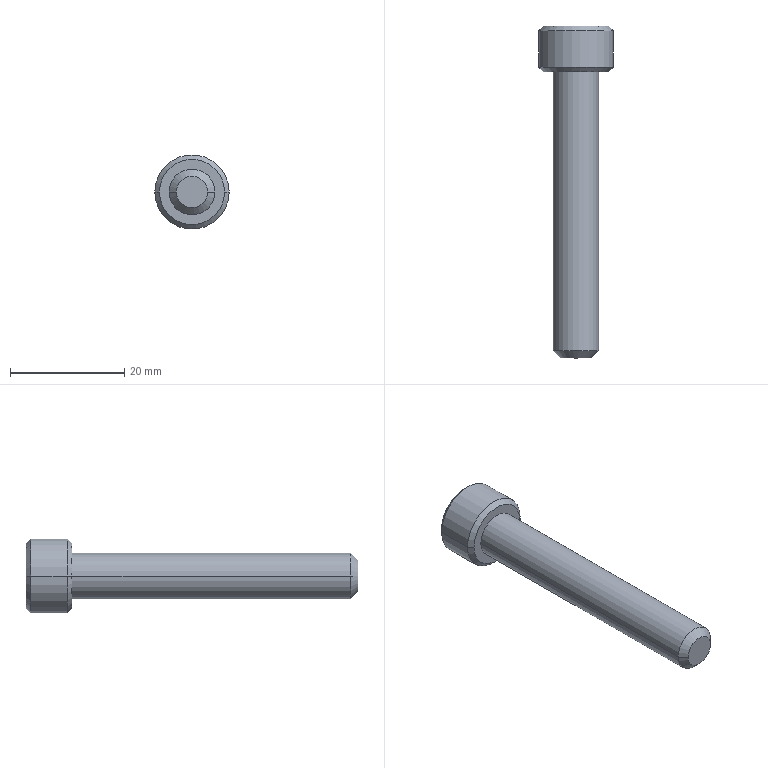Part | STEP file | BB62-M8-50L | 1 solid | 27 faces | box 13 x 58 x 13 mm | volume 3386 mm3 | plane 15 | cone 8 | cylinder 4 | commonest cylinder face diameters 8 x2 13 x2
STEP:
#1=CARTESIAN_POINT('',(0.,2.02,0.));
#2=VERTEX_POINT('',#1);
#3=CARTESIAN_POINT('',(3.43,4.,0.));
#4=VERTEX_POINT('',#3);
#5=CARTESIAN_POINT('',(0.,2.02,0.));
#6=DIRECTION('',(0.866,0.5,0.));
#7=VECTOR('',#6,1000.);
#8=LINE('',#5,#7);
#9=EDGE_CURVE('',#2,#4,#8,.T.);
#10=ORIENTED_EDGE('',*,*,#9,.F.);
#11=CARTESIAN_POINT('',(-3.43,4.,0.));
#12=VERTEX_POINT('',#11);
#13=CARTESIAN_POINT('',(0.,2.02,0.));
#14=DIRECTION('',(-0.866,0.5,0.));
#15=VECTOR('',#14,1000.);
#16=LINE('',#13,#15);
#17=EDGE_CURVE('',#2,#12,#16,.T.);
#18=ORIENTED_EDGE('',*,*,#17,.T.);
#19=CARTESIAN_POINT('',(-2.97,4.,1.715));
#20=VERTEX_POINT('',#19);
#21=CARTESIAN_POINT('',(0.,4.,0.));
#22=DIRECTION('',(0.,-1.,0.));
#23=DIRECTION('',(-1.,0.,0.));
#24=AXIS2_PLACEMENT_3D('',#21,#22,#23);
#25=CIRCLE('',#24,3.43);
#26=EDGE_CURVE('',#20,#12,#25,.T.);
#27=ORIENTED_EDGE('',*,*,#26,.F.);
#28=CARTESIAN_POINT('',(0.,4.,3.43));
#29=VERTEX_POINT('',#28);
#30=CARTESIAN_POINT('',(0.,4.,0.));
#31=DIRECTION('',(0.,-1.,0.));
#32=DIRECTION('',(-1.,0.,0.));
#33=AXIS2_PLACEMENT_3D('',#30,#31,#32);
#34=CIRCLE('',#33,3.43);
#35=EDGE_CURVE('',#29,#20,#34,.T.);
#36=ORIENTED_EDGE('',*,*,#35,.F.);
#37=CARTESIAN_POINT('',(2.97,4.,1.715));
#38=VERTEX_POINT('',#37);
#39=CARTESIAN_POINT('',(0.,4.,0.));
#40=DIRECTION('',(0.,-1.,0.));
#41=DIRECTION('',(-1.,0.,0.));
#42=AXIS2_PLACEMENT_3D('',#39,#40,#41);
#43=CIRCLE('',#42,3.43);
#44=EDGE_CURVE('',#38,#29,#43,.T.);
#45=ORIENTED_EDGE('',*,*,#44,.F.);
#46=CARTESIAN_POINT('',(0.,4.,0.));
#47=DIRECTION('',(0.,-1.,0.));
#48=DIRECTION('',(-1.,0.,0.));
#49=AXIS2_PLACEMENT_3D('',#46,#47,#48);
#50=CIRCLE('',#49,3.43);
#51=EDGE_CURVE('',#4,#38,#50,.T.);
#52=ORIENTED_EDGE('',*,*,#51,.F.);
#53=EDGE_LOOP('',(#10,#18,#27,#36,#45,#52));
#54=FACE_OUTER_BOUND('',#53,.T.);
#55=CARTESIAN_POINT('',(0.,1002.02,0.));
#56=DIRECTION('',(0.,1.,0.));
#57=DIRECTION('',(1.,0.,0.));
#58=AXIS2_PLACEMENT_3D('',#55,#56,#57);
#59=CONICAL_SURFACE('',#58,1732.051,1.047);
#60=ADVANCED_FACE('',(#54),#59,.F.);
#61=CARTESIAN_POINT('',(2.75,-50.,0.));
#62=VERTEX_POINT('',#61);
#63=CARTESIAN_POINT('',(-2.75,-50.,0.));
#64=VERTEX_POINT('',#63);
#65=CARTESIAN_POINT('',(0.,-50.,0.));
#66=DIRECTION('',(0.,1.,0.));
#67=DIRECTION('',(1.,0.,0.));
#68=AXIS2_PLACEMENT_3D('',#65,#66,#67);
#69=CIRCLE('',#68,2.75);
#70=EDGE_CURVE('',#62,#64,#69,.T.);
#71=ORIENTED_EDGE('',*,*,#70,.T.);
#72=CARTESIAN_POINT('',(-4.,-48.75,0.));
#73=VERTEX_POINT('',#72);
#74=CARTESIAN_POINT('',(-2.75,-50.,0.));
#75=DIRECTION('',(-0.7071,0.7071,0.));
#76=VECTOR('',#75,1000.);
#77=LINE('',#74,#76);
#78=EDGE_CURVE('',#64,#73,#77,.T.);
#79=ORIENTED_EDGE('',*,*,#78,.T.);
#80=CARTESIAN_POINT('',(4.,-48.75,0.));
#81=VERTEX_POINT('',#80);
#82=CARTESIAN_POINT('',(0.,-48.75,0.));
#83=DIRECTION('',(0.,-1.,0.));
#84=DIRECTION('',(-1.,0.,0.));
#85=AXIS2_PLACEMENT_3D('',#82,#83,#84);
#86=CIRCLE('',#85,4.);
#87=EDGE_CURVE('',#73,#81,#86,.T.);
#88=ORIENTED_EDGE('',*,*,#87,.T.);
#89=CARTESIAN_POINT('',(2.75,-50.,0.));
#90=DIRECTION('',(0.7071,0.7071,0.));
#91=VECTOR('',#90,1000.);
#92=LINE('',#89,#91);
#93=EDGE_CURVE('',#62,#81,#92,.T.);
#94=ORIENTED_EDGE('',*,*,#93,.F.);
#95=EDGE_LOOP('',(#71,#79,#88,#94));
#96=FACE_OUTER_BOUND('',#95,.T.);
#97=CARTESIAN_POINT('',(0.,-50.,0.));
#98=DIRECTION('',(0.,1.,0.));
#99=DIRECTION('',(1.,0.,0.));
#100=AXIS2_PLACEMENT_3D('',#97,#98,#99);
#101=CONICAL_SURFACE('',#100,2.75,0.7854);
#102=ADVANCED_FACE('',(#96),#101,.T.);
#103=ORIENTED_EDGE('',*,*,#87,.F.);
#104=CARTESIAN_POINT('',(-4.,0.,0.));
#105=VERTEX_POINT('',#104);
#106=CARTESIAN_POINT('',(-4.,-48.75,0.));
#107=DIRECTION('',(0.,1.,0.));
#108=VECTOR('',#107,1000.);
#109=LINE('',#106,#108);
#110=EDGE_CURVE('',#73,#105,#109,.T.);
#111=ORIENTED_EDGE('',*,*,#110,.T.);
#112=CARTESIAN_POINT('',(4.,0.,0.));
#113=VERTEX_POINT('',#112);
#114=CARTESIAN_POINT('',(0.,0.,0.));
#115=DIRECTION('',(0.,-1.,0.));
#116=DIRECTION('',(-1.,0.,0.));
#117=AXIS2_PLACEMENT_3D('',#114,#115,#116);
#118=CIRCLE('',#117,4.);
#119=EDGE_CURVE('',#105,#113,#118,.T.);
#120=ORIENTED_EDGE('',*,*,#119,.T.);
#121=CARTESIAN_POINT('',(4.,-48.75,0.));
#122=DIRECTION('',(0.,1.,0.));
#123=VECTOR('',#122,1000.);
#124=LINE('',#121,#123);
#125=EDGE_CURVE('',#81,#113,#124,.T.);
#126=ORIENTED_EDGE('',*,*,#125,.F.);
#127=EDGE_LOOP('',(#103,#111,#120,#126));
#128=FACE_OUTER_BOUND('',#127,.T.);
#129=CARTESIAN_POINT('',(0.,-48.75,0.));
#130=DIRECTION('',(0.,1.,0.));
#131=DIRECTION('',(1.,0.,0.));
#132=AXIS2_PLACEMENT_3D('',#129,#130,#131);
#133=CYLINDRICAL_SURFACE('',#132,4.);
#134=ADVANCED_FACE('',(#128),#133,.T.);
#135=CARTESIAN_POINT('',(-5.7,8.,0.));
#136=VERTEX_POINT('',#135);
#137=CARTESIAN_POINT('',(5.7,8.,0.));
#138=VERTEX_POINT('',#137);
#139=CARTESIAN_POINT('',(0.,8.,0.));
#140=DIRECTION('',(0.,-1.,0.));
#141=DIRECTION('',(-1.,0.,0.));
#142=AXIS2_PLACEMENT_3D('',#139,#140,#141);
#143=CIRCLE('',#142,5.7);
#144=EDGE_CURVE('',#136,#138,#143,.T.);
#145=ORIENTED_EDGE('',*,*,#144,.T.);
#146=CARTESIAN_POINT('',(6.5,7.2,0.));
#147=VERTEX_POINT('',#146);
#148=CARTESIAN_POINT('',(6.5,7.2,0.));
#149=DIRECTION('',(0.7071,-0.7071,0.));
#150=VECTOR('',#149,1000.);
#151=LINE('',#148,#150);
#152=EDGE_CURVE('',#138,#147,#151,.T.);
#153=ORIENTED_EDGE('',*,*,#152,.T.);
#154=CARTESIAN_POINT('',(-6.5,7.2,0.));
#155=VERTEX_POINT('',#154);
#156=CARTESIAN_POINT('',(0.,7.2,0.));
#157=DIRECTION('',(0.,-1.,0.));
#158=DIRECTION('',(-1.,0.,0.));
#159=AXIS2_PLACEMENT_3D('',#156,#157,#158);
#160=CIRCLE('',#159,6.5);
#161=EDGE_CURVE('',#155,#147,#160,.T.);
#162=ORIENTED_EDGE('',*,*,#161,.F.);
#163=CARTESIAN_POINT('',(-6.5,7.2,0.));
#164=DIRECTION('',(-0.7071,-0.7071,0.));
#165=VECTOR('',#164,1000.);
#166=LINE('',#163,#165);
#167=EDGE_CURVE('',#136,#155,#166,.T.);
#168=ORIENTED_EDGE('',*,*,#167,.F.);
#169=EDGE_LOOP('',(#145,#153,#162,#168));
#170=FACE_OUTER_BOUND('',#169,.T.);
#171=CARTESIAN_POINT('',(0.,7.2,0.));
#172=DIRECTION('',(0.,-1.,0.));
#173=DIRECTION('',(-1.,0.,0.));
#174=AXIS2_PLACEMENT_3D('',#171,#172,#173);
#175=CONICAL_SURFACE('',#174,6.5,0.7854);
#176=ADVANCED_FACE('',(#170),#175,.T.);
#177=ORIENTED_EDGE('',*,*,#161,.T.);
#178=CARTESIAN_POINT('',(6.5,0.8,0.));
#179=VERTEX_POINT('',#178);
#180=CARTESIAN_POINT('',(6.5,1.62,0.));
#181=DIRECTION('',(0.,-1.,0.));
#182=VECTOR('',#181,1000.);
#183=LINE('',#180,#182);
#184=EDGE_CURVE('',#147,#179,#183,.T.);
#185=ORIENTED_EDGE('',*,*,#184,.T.);
#186=CARTESIAN_POINT('',(-6.5,0.8,0.));
#187=VERTEX_POINT('',#186);
#188=CARTESIAN_POINT('',(0.,0.8,0.));
#189=DIRECTION('',(0.,-1.,0.));
#190=DIRECTION('',(-1.,0.,0.));
#191=AXIS2_PLACEMENT_3D('',#188,#189,#190);
#192=CIRCLE('',#191,6.5);
#193=EDGE_CURVE('',#187,#179,#192,.T.);
#194=ORIENTED_EDGE('',*,*,#193,.F.);
#195=CARTESIAN_POINT('',(-6.5,1.62,0.));
#196=DIRECTION('',(0.,-1.,0.));
#197=VECTOR('',#196,1000.);
#198=LINE('',#195,#197);
#199=EDGE_CURVE('',#155,#187,#198,.T.);
#200=ORIENTED_EDGE('',*,*,#199,.F.);
#201=EDGE_LOOP('',(#177,#185,#194,#200));
#202=FACE_OUTER_BOUND('',#201,.T.);
#203=CARTESIAN_POINT('',(0.,1.62,0.));
#204=DIRECTION('',(0.,-1.,0.));
#205=DIRECTION('',(-1.,0.,0.));
#206=AXIS2_PLACEMENT_3D('',#203,#204,#205);
#207=CYLINDRICAL_SURFACE('',#206,6.5);
#208=ADVANCED_FACE('',(#202),#207,.T.);
#209=CARTESIAN_POINT('',(-5.7,0.,0.));
#210=VERTEX_POINT('',#209);
#211=CARTESIAN_POINT('',(5.7,0.,0.));
#212=VERTEX_POINT('',#211);
#213=CARTESIAN_POINT('',(0.,0.,0.));
#214=DIRECTION('',(0.,-1.,0.));
#215=DIRECTION('',(-1.,0.,0.));
#216=AXIS2_PLACEMENT_3D('',#213,#214,#215);
#217=CIRCLE('',#216,5.7);
#218=EDGE_CURVE('',#210,#212,#217,.T.);
#219=ORIENTED_EDGE('',*,*,#218,.F.);
#220=CARTESIAN_POINT('',(-5.7,0.,0.));
#221=DIRECTION('',(-0.7071,0.7071,0.));
#222=VECTOR('',#221,1000.);
#223=LINE('',#220,#222);
#224=EDGE_CURVE('',#210,#187,#223,.T.);
#225=ORIENTED_EDGE('',*,*,#224,.T.);
#226=ORIENTED_EDGE('',*,*,#193,.T.);
#227=CARTESIAN_POINT('',(5.7,0.,0.));
#228=DIRECTION('',(0.7071,0.7071,0.));
#229=VECTOR('',#228,1000.);
#230=LINE('',#227,#229);
#231=EDGE_CURVE('',#212,#179,#230,.T.);
#232=ORIENTED_EDGE('',*,*,#231,.F.);
#233=EDGE_LOOP('',(#219,#225,#226,#232));
#234=FACE_OUTER_BOUND('',#233,.T.);
#235=CARTESIAN_POINT('',(0.,0.,0.));
#236=DIRECTION('',(0.,1.,0.));
#237=DIRECTION('',(1.,0.,0.));
#238=AXIS2_PLACEMENT_3D('',#235,#236,#237);
#239=CONICAL_SURFACE('',#238,5.7,0.7854);
#240=ADVANCED_FACE('',(#234),#239,.T.);
#241=ORIENTED_EDGE('',*,*,#144,.F.);
#242=CARTESIAN_POINT('',(0.,8.,0.));
#243=DIRECTION('',(0.,-1.,0.));
#244=DIRECTION('',(-1.,0.,0.));
#245=AXIS2_PLACEMENT_3D('',#242,#243,#244);
#246=CIRCLE('',#245,5.7);
#247=EDGE_CURVE('',#138,#136,#246,.T.);
#248=ORIENTED_EDGE('',*,*,#247,.F.);
#249=EDGE_LOOP('',(#241,#248));
#250=FACE_OUTER_BOUND('',#249,.T.);
#251=CARTESIAN_POINT('',(0.,8.,-3.43));
#252=VERTEX_POINT('',#251);
#253=CARTESIAN_POINT('',(-2.97,8.,-1.715));
#254=VERTEX_POINT('',#253);
#255=CARTESIAN_POINT('',(0.,8.,-3.43));
#256=DIRECTION('',(-0.866,0.,0.5));
#257=VECTOR('',#256,1000.);
#258=LINE('',#255,#257);
#259=EDGE_CURVE('',#252,#254,#258,.T.);
#260=ORIENTED_EDGE('',*,*,#259,.F.);
#261=CARTESIAN_POINT('',(2.97,8.,-1.715));
#262=VERTEX_POINT('',#261);
#263=CARTESIAN_POINT('',(2.97,8.,-1.715));
#264=DIRECTION('',(-0.866,0.,-0.5));
#265=VECTOR('',#264,1000.);
#266=LINE('',#263,#265);
#267=EDGE_CURVE('',#262,#252,#266,.T.);
#268=ORIENTED_EDGE('',*,*,#267,.F.);
#269=CARTESIAN_POINT('',(2.97,8.,1.715));
#270=VERTEX_POINT('',#269);
#271=CARTESIAN_POINT('',(2.97,8.,1.715));
#272=DIRECTION('',(0.,0.,-1.));
#273=VECTOR('',#272,1000.);
#274=LINE('',#271,#273);
#275=EDGE_CURVE('',#270,#262,#274,.T.);
#276=ORIENTED_EDGE('',*,*,#275,.F.);
#277=CARTESIAN_POINT('',(0.,8.,3.43));
#278=VERTEX_POINT('',#277);
#279=CARTESIAN_POINT('',(0.,8.,3.43));
#280=DIRECTION('',(0.866,0.,-0.5));
#281=VECTOR('',#280,1000.);
#282=LINE('',#279,#281);
#283=EDGE_CURVE('',#278,#270,#282,.T.);
#284=ORIENTED_EDGE('',*,*,#283,.F.);
#285=CARTESIAN_POINT('',(-2.97,8.,1.715));
#286=VERTEX_POINT('',#285);
#287=CARTESIAN_POINT('',(-2.97,8.,1.715));
#288=DIRECTION('',(0.866,0.,0.5));
#289=VECTOR('',#288,1000.);
#290=LINE('',#287,#289);
#291=EDGE_CURVE('',#286,#278,#290,.T.);
#292=ORIENTED_EDGE('',*,*,#291,.F.);
#293=CARTESIAN_POINT('',(-2.97,8.,-1.715));
#294=DIRECTION('',(0.,0.,1.));
#295=VECTOR('',#294,1000.);
#296=LINE('',#293,#295);
#297=EDGE_CURVE('',#254,#286,#296,.T.);
#298=ORIENTED_EDGE('',*,*,#297,.F.);
#299=EDGE_LOOP('',(#260,#268,#276,#284,#292,#298));
#300=FACE_BOUND('',#299,.T.);
#301=CARTESIAN_POINT('',(5.7,8.,0.));
#302=DIRECTION('',(0.,1.,0.));
#303=DIRECTION('',(1.,0.,0.));
#304=AXIS2_PLACEMENT_3D('',#301,#302,#303);
#305=PLANE('',#304);
#306=ADVANCED_FACE('',(#250,#300),#305,.T.);
#307=CARTESIAN_POINT('',(0.,0.,0.));
#308=DIRECTION('',(0.,-1.,0.));
#309=DIRECTION('',(-1.,0.,0.));
#310=AXIS2_PLACEMENT_3D('',#307,#308,#309);
#311=CIRCLE('',#310,4.);
#312=EDGE_CURVE('',#113,#105,#311,.T.);
#313=ORIENTED_EDGE('',*,*,#312,.F.);
#314=ORIENTED_EDGE('',*,*,#119,.F.);
#315=EDGE_LOOP('',(#313,#314));
#316=FACE_BOUND('',#315,.T.);
#317=CARTESIAN_POINT('',(0.,0.,0.));
#318=DIRECTION('',(0.,-1.,0.));
#319=DIRECTION('',(-1.,0.,0.));
#320=AXIS2_PLACEMENT_3D('',#317,#318,#319);
#321=CIRCLE('',#320,5.7);
#322=EDGE_CURVE('',#212,#210,#321,.T.);
#323=ORIENTED_EDGE('',*,*,#322,.T.);
#324=ORIENTED_EDGE('',*,*,#218,.T.);
#325=EDGE_LOOP('',(#323,#324));
#326=FACE_OUTER_BOUND('',#325,.T.);
#327=CARTESIAN_POINT('',(0.,0.,0.));
#328=DIRECTION('',(0.,-1.,0.));
#329=DIRECTION('',(-1.,0.,0.));
#330=AXIS2_PLACEMENT_3D('',#327,#328,#329);
#331=PLANE('',#330);
#332=ADVANCED_FACE('',(#316,#326),#331,.T.);
#333=ORIENTED_EDGE('',*,*,#224,.F.);
#334=ORIENTED_EDGE('',*,*,#322,.F.);
#335=ORIENTED_EDGE('',*,*,#231,.T.);
#336=CARTESIAN_POINT('',(0.,0.8,0.));
#337=DIRECTION('',(0.,-1.,0.));
#338=DIRECTION('',(-1.,0.,0.));
#339=AXIS2_PLACEMENT_3D('',#336,#337,#338);
#340=CIRCLE('',#339,6.5);
#341=EDGE_CURVE('',#179,#187,#340,.T.);
#342=ORIENTED_EDGE('',*,*,#341,.T.);
#343=EDGE_LOOP('',(#333,#334,#335,#342));
#344=FACE_OUTER_BOUND('',#343,.T.);
#345=CARTESIAN_POINT('',(0.,0.,0.));
#346=DIRECTION('',(0.,1.,0.));
#347=DIRECTION('',(1.,0.,0.));
#348=AXIS2_PLACEMENT_3D('',#345,#346,#347);
#349=CONICAL_SURFACE('',#348,5.7,0.7854);
#350=ADVANCED_FACE('',(#344),#349,.T.);
#351=ORIENTED_EDGE('',*,*,#184,.F.);
#352=CARTESIAN_POINT('',(0.,7.2,0.));
#353=DIRECTION('',(0.,-1.,0.));
#354=DIRECTION('',(-1.,0.,0.));
#355=AXIS2_PLACEMENT_3D('',#352,#353,#354);
#356=CIRCLE('',#355,6.5);
#357=EDGE_CURVE('',#147,#155,#356,.T.);
#358=ORIENTED_EDGE('',*,*,#357,.T.);
#359=ORIENTED_EDGE('',*,*,#199,.T.);
#360=ORIENTED_EDGE('',*,*,#341,.F.);
#361=EDGE_LOOP('',(#351,#358,#359,#360));
#362=FACE_OUTER_BOUND('',#361,.T.);
#363=CARTESIAN_POINT('',(0.,1.62,0.));
#364=DIRECTION('',(0.,-1.,0.));
#365=DIRECTION('',(-1.,0.,0.));
#366=AXIS2_PLACEMENT_3D('',#363,#364,#365);
#367=CYLINDRICAL_SURFACE('',#366,6.5);
#368=ADVANCED_FACE('',(#362),#367,.T.);
#369=ORIENTED_EDGE('',*,*,#152,.F.);
#370=ORIENTED_EDGE('',*,*,#247,.T.);
#371=ORIENTED_EDGE('',*,*,#167,.T.);
#372=ORIENTED_EDGE('',*,*,#357,.F.);
#373=EDGE_LOOP('',(#369,#370,#371,#372));
#374=FACE_OUTER_BOUND('',#373,.T.);
#375=CARTESIAN_POINT('',(0.,7.2,0.));
#376=DIRECTION('',(0.,-1.,0.));
#377=DIRECTION('',(-1.,0.,0.));
#378=AXIS2_PLACEMENT_3D('',#375,#376,#377);
#379=CONICAL_SURFACE('',#378,6.5,0.7854);
#380=ADVANCED_FACE('',(#374),#379,.T.);
#381=ORIENTED_EDGE('',*,*,#110,.F.);
#382=CARTESIAN_POINT('',(0.,-48.75,0.));
#383=DIRECTION('',(0.,-1.,0.));
#384=DIRECTION('',(-1.,0.,0.));
#385=AXIS2_PLACEMENT_3D('',#382,#383,#384);
#386=CIRCLE('',#385,4.);
#387=EDGE_CURVE('',#81,#73,#386,.T.);
#388=ORIENTED_EDGE('',*,*,#387,.F.);
#389=ORIENTED_EDGE('',*,*,#125,.T.);
#390=ORIENTED_EDGE('',*,*,#312,.T.);
#391=EDGE_LOOP('',(#381,#388,#389,#390));
#392=FACE_OUTER_BOUND('',#391,.T.);
#393=CARTESIAN_POINT('',(0.,-48.75,0.));
#394=DIRECTION('',(0.,1.,0.));
#395=DIRECTION('',(1.,0.,0.));
#396=AXIS2_PLACEMENT_3D('',#393,#394,#395);
#397=CYLINDRICAL_SURFACE('',#396,4.);
#398=ADVANCED_FACE('',(#392),#397,.T.);
#399=ORIENTED_EDGE('',*,*,#70,.F.);
#400=CARTESIAN_POINT('',(0.,-50.,0.));
#401=DIRECTION('',(0.,1.,0.));
#402=DIRECTION('',(1.,0.,0.));
#403=AXIS2_PLACEMENT_3D('',#400,#401,#402);
#404=CIRCLE('',#403,2.75);
#405=EDGE_CURVE('',#64,#62,#404,.T.);
#406=ORIENTED_EDGE('',*,*,#405,.F.);
#407=EDGE_LOOP('',(#399,#406));
#408=FACE_OUTER_BOUND('',#407,.T.);
#409=CARTESIAN_POINT('',(0.,-50.,0.));
#410=DIRECTION('',(0.,-1.,0.));
#411=DIRECTION('',(-1.,0.,0.));
#412=AXIS2_PLACEMENT_3D('',#409,#410,#411);
#413=PLANE('',#412);
#414=ADVANCED_FACE('',(#408),#413,.T.);
#415=ORIENTED_EDGE('',*,*,#78,.F.);
#416=ORIENTED_EDGE('',*,*,#405,.T.);
#417=ORIENTED_EDGE('',*,*,#93,.T.);
#418=ORIENTED_EDGE('',*,*,#387,.T.);
#419=EDGE_LOOP('',(#415,#416,#417,#418));
#420=FACE_OUTER_BOUND('',#419,.T.);
#421=CARTESIAN_POINT('',(0.,-50.,0.));
#422=DIRECTION('',(0.,1.,0.));
#423=DIRECTION('',(1.,0.,0.));
#424=AXIS2_PLACEMENT_3D('',#421,#422,#423);
#425=CONICAL_SURFACE('',#424,2.75,0.7854);
#426=ADVANCED_FACE('',(#420),#425,.T.);
#427=CARTESIAN_POINT('',(2.97,4.,-1.715));
#428=VERTEX_POINT('',#427);
#429=CARTESIAN_POINT('',(0.,4.,-3.43));
#430=VERTEX_POINT('',#429);
#431=CARTESIAN_POINT('',(2.97,4.,-1.715));
#432=DIRECTION('',(-0.866,0.,-0.5));
#433=VECTOR('',#432,1000.);
#434=LINE('',#431,#433);
#435=EDGE_CURVE('',#428,#430,#434,.T.);
#436=ORIENTED_EDGE('',*,*,#435,.F.);
#437=CARTESIAN_POINT('',(2.97,8.,-1.715));
#438=DIRECTION('',(0.,-1.,0.));
#439=VECTOR('',#438,1000.);
#440=LINE('',#437,#439);
#441=EDGE_CURVE('',#262,#428,#440,.T.);
#442=ORIENTED_EDGE('',*,*,#441,.F.);
#443=ORIENTED_EDGE('',*,*,#267,.T.);
#444=CARTESIAN_POINT('',(0.,8.,-3.43));
#445=DIRECTION('',(0.,-1.,0.));
#446=VECTOR('',#445,1000.);
#447=LINE('',#444,#446);
#448=EDGE_CURVE('',#252,#430,#447,.T.);
#449=ORIENTED_EDGE('',*,*,#448,.T.);
#450=EDGE_LOOP('',(#436,#442,#443,#449));
#451=FACE_OUTER_BOUND('',#450,.T.);
#452=CARTESIAN_POINT('',(2.97,8.,-1.715));
#453=DIRECTION('',(-0.5,0.,0.866));
#454=DIRECTION('',(0.866,0.,0.5));
#455=AXIS2_PLACEMENT_3D('',#452,#453,#454);
#456=PLANE('',#455);
#457=ADVANCED_FACE('',(#451),#456,.T.);
#458=CARTESIAN_POINT('',(-2.97,4.,-1.715));
#459=VERTEX_POINT('',#458);
#460=CARTESIAN_POINT('',(0.,4.,-3.43));
#461=DIRECTION('',(-0.866,0.,0.5));
#462=VECTOR('',#461,1000.);
#463=LINE('',#460,#462);
#464=EDGE_CURVE('',#430,#459,#463,.T.);
#465=ORIENTED_EDGE('',*,*,#464,.F.);
#466=ORIENTED_EDGE('',*,*,#448,.F.);
#467=ORIENTED_EDGE('',*,*,#259,.T.);
#468=CARTESIAN_POINT('',(-2.97,8.,-1.715));
#469=DIRECTION('',(0.,-1.,0.));
#470=VECTOR('',#469,1000.);
#471=LINE('',#468,#470);
#472=EDGE_CURVE('',#254,#459,#471,.T.);
#473=ORIENTED_EDGE('',*,*,#472,.T.);
#474=EDGE_LOOP('',(#465,#466,#467,#473));
#475=FACE_OUTER_BOUND('',#474,.T.);
#476=CARTESIAN_POINT('',(0.,8.,-3.43));
#477=DIRECTION('',(0.5,0.,0.866));
#478=DIRECTION('',(0.866,0.,-0.5));
#479=AXIS2_PLACEMENT_3D('',#476,#477,#478);
#480=PLANE('',#479);
#481=ADVANCED_FACE('',(#475),#480,.T.);
#482=CARTESIAN_POINT('',(-2.97,4.,-1.715));
#483=DIRECTION('',(0.,0.,1.));
#484=VECTOR('',#483,1000.);
#485=LINE('',#482,#484);
#486=EDGE_CURVE('',#459,#20,#485,.T.);
#487=ORIENTED_EDGE('',*,*,#486,.F.);
#488=ORIENTED_EDGE('',*,*,#472,.F.);
#489=ORIENTED_EDGE('',*,*,#297,.T.);
#490=CARTESIAN_POINT('',(-2.97,8.,1.715));
#491=DIRECTION('',(0.,-1.,0.));
#492=VECTOR('',#491,1000.);
#493=LINE('',#490,#492);
#494=EDGE_CURVE('',#286,#20,#493,.T.);
#495=ORIENTED_EDGE('',*,*,#494,.T.);
#496=EDGE_LOOP('',(#487,#488,#489,#495));
#497=FACE_OUTER_BOUND('',#496,.T.);
#498=CARTESIAN_POINT('',(-2.97,8.,-1.715));
#499=DIRECTION('',(1.,0.,0.));
#500=DIRECTION('',(0.,0.,-1.));
#501=AXIS2_PLACEMENT_3D('',#498,#499,#500);
#502=PLANE('',#501);
#503=ADVANCED_FACE('',(#497),#502,.T.);
#504=CARTESIAN_POINT('',(-2.97,4.,1.715));
#505=DIRECTION('',(0.866,0.,0.5));
#506=VECTOR('',#505,1000.);
#507=LINE('',#504,#506);
#508=EDGE_CURVE('',#20,#29,#507,.T.);
#509=ORIENTED_EDGE('',*,*,#508,.F.);
#510=ORIENTED_EDGE('',*,*,#494,.F.);
#511=ORIENTED_EDGE('',*,*,#291,.T.);
#512=CARTESIAN_POINT('',(0.,8.,3.43));
#513=DIRECTION('',(0.,-1.,0.));
#514=VECTOR('',#513,1000.);
#515=LINE('',#512,#514);
#516=EDGE_CURVE('',#278,#29,#515,.T.);
#517=ORIENTED_EDGE('',*,*,#516,.T.);
#518=EDGE_LOOP('',(#509,#510,#511,#517));
#519=FACE_OUTER_BOUND('',#518,.T.);
#520=CARTESIAN_POINT('',(-2.97,8.,1.715));
#521=DIRECTION('',(0.5,0.,-0.866));
#522=DIRECTION('',(-0.866,0.,-0.5));
#523=AXIS2_PLACEMENT_3D('',#520,#521,#522);
#524=PLANE('',#523);
#525=ADVANCED_FACE('',(#519),#524,.T.);
#526=CARTESIAN_POINT('',(0.,4.,3.43));
#527=DIRECTION('',(0.866,0.,-0.5));
#528=VECTOR('',#527,1000.);
#529=LINE('',#526,#528);
#530=EDGE_CURVE('',#29,#38,#529,.T.);
#531=ORIENTED_EDGE('',*,*,#530,.F.);
#532=ORIENTED_EDGE('',*,*,#516,.F.);
#533=ORIENTED_EDGE('',*,*,#283,.T.);
#534=CARTESIAN_POINT('',(2.97,8.,1.715));
#535=DIRECTION('',(0.,-1.,0.));
#536=VECTOR('',#535,1000.);
#537=LINE('',#534,#536);
#538=EDGE_CURVE('',#270,#38,#537,.T.);
#539=ORIENTED_EDGE('',*,*,#538,.T.);
#540=EDGE_LOOP('',(#531,#532,#533,#539));
#541=FACE_OUTER_BOUND('',#540,.T.);
#542=CARTESIAN_POINT('',(0.,8.,3.43));
#543=DIRECTION('',(-0.5,0.,-0.866));
#544=DIRECTION('',(-0.866,0.,0.5));
#545=AXIS2_PLACEMENT_3D('',#542,#543,#544);
#546=PLANE('',#545);
#547=ADVANCED_FACE('',(#541),#546,.T.);
#548=CARTESIAN_POINT('',(2.97,4.,1.715));
#549=DIRECTION('',(0.,0.,-1.));
#550=VECTOR('',#549,1000.);
#551=LINE('',#548,#550);
#552=EDGE_CURVE('',#38,#428,#551,.T.);
#553=ORIENTED_EDGE('',*,*,#552,.F.);
#554=ORIENTED_EDGE('',*,*,#538,.F.);
#555=ORIENTED_EDGE('',*,*,#275,.T.);
#556=ORIENTED_EDGE('',*,*,#441,.T.);
#557=EDGE_LOOP('',(#553,#554,#555,#556));
#558=FACE_OUTER_BOUND('',#557,.T.);
#559=CARTESIAN_POINT('',(2.97,8.,1.715));
#560=DIRECTION('',(-1.,0.,0.));
#561=DIRECTION('',(0.,0.,1.));
#562=AXIS2_PLACEMENT_3D('',#559,#560,#561);
#563=PLANE('',#562);
#564=ADVANCED_FACE('',(#558),#563,.T.);
#565=ORIENTED_EDGE('',*,*,#435,.T.);
#566=CARTESIAN_POINT('',(0.,4.,0.));
#567=DIRECTION('',(0.,-1.,0.));
#568=DIRECTION('',(-1.,0.,0.));
#569=AXIS2_PLACEMENT_3D('',#566,#567,#568);
#570=CIRCLE('',#569,3.43);
#571=EDGE_CURVE('',#430,#428,#570,.T.);
#572=ORIENTED_EDGE('',*,*,#571,.T.);
#573=EDGE_LOOP('',(#565,#572));
#574=FACE_OUTER_BOUND('',#573,.T.);
#575=CARTESIAN_POINT('',(0.,4.,0.));
#576=DIRECTION('',(0.,1.,0.));
#577=DIRECTION('',(1.,0.,0.));
#578=AXIS2_PLACEMENT_3D('',#575,#576,#577);
#579=PLANE('',#578);
#580=ADVANCED_FACE('',(#574),#579,.F.);
#581=ORIENTED_EDGE('',*,*,#552,.T.);
#582=CARTESIAN_POINT('',(0.,4.,0.));
#583=DIRECTION('',(0.,-1.,0.));
#584=DIRECTION('',(-1.,0.,0.));
#585=AXIS2_PLACEMENT_3D('',#582,#583,#584);
#586=CIRCLE('',#585,3.43);
#587=EDGE_CURVE('',#428,#4,#586,.T.);
#588=ORIENTED_EDGE('',*,*,#587,.T.);
#589=ORIENTED_EDGE('',*,*,#51,.T.);
#590=EDGE_LOOP('',(#581,#588,#589));
#591=FACE_OUTER_BOUND('',#590,.T.);
#592=CARTESIAN_POINT('',(0.,4.,0.));
#593=DIRECTION('',(0.,1.,0.));
#594=DIRECTION('',(1.,0.,0.));
#595=AXIS2_PLACEMENT_3D('',#592,#593,#594);
#596=PLANE('',#595);
#597=ADVANCED_FACE('',(#591),#596,.F.);
#598=ORIENTED_EDGE('',*,*,#530,.T.);
#599=ORIENTED_EDGE('',*,*,#44,.T.);
#600=EDGE_LOOP('',(#598,#599));
#601=FACE_OUTER_BOUND('',#600,.T.);
#602=CARTESIAN_POINT('',(0.,4.,0.));
#603=DIRECTION('',(0.,1.,0.));
#604=DIRECTION('',(1.,0.,0.));
#605=AXIS2_PLACEMENT_3D('',#602,#603,#604);
#606=PLANE('',#605);
#607=ADVANCED_FACE('',(#601),#606,.F.);
#608=ORIENTED_EDGE('',*,*,#508,.T.);
#609=ORIENTED_EDGE('',*,*,#35,.T.);
#610=EDGE_LOOP('',(#608,#609));
#611=FACE_OUTER_BOUND('',#610,.T.);
#612=CARTESIAN_POINT('',(0.,4.,0.));
#613=DIRECTION('',(0.,1.,0.));
#614=DIRECTION('',(1.,0.,0.));
#615=AXIS2_PLACEMENT_3D('',#612,#613,#614);
#616=PLANE('',#615);
#617=ADVANCED_FACE('',(#611),#616,.F.);
#618=ORIENTED_EDGE('',*,*,#486,.T.);
#619=ORIENTED_EDGE('',*,*,#26,.T.);
#620=CARTESIAN_POINT('',(0.,4.,0.));
#621=DIRECTION('',(0.,-1.,0.));
#622=DIRECTION('',(-1.,0.,0.));
#623=AXIS2_PLACEMENT_3D('',#620,#621,#622);
#624=CIRCLE('',#623,3.43);
#625=EDGE_CURVE('',#12,#459,#624,.T.);
#626=ORIENTED_EDGE('',*,*,#625,.T.);
#627=EDGE_LOOP('',(#618,#619,#626));
#628=FACE_OUTER_BOUND('',#627,.T.);
#629=CARTESIAN_POINT('',(0.,4.,0.));
#630=DIRECTION('',(0.,1.,0.));
#631=DIRECTION('',(1.,0.,0.));
#632=AXIS2_PLACEMENT_3D('',#629,#630,#631);
#633=PLANE('',#632);
#634=ADVANCED_FACE('',(#628),#633,.F.);
#635=ORIENTED_EDGE('',*,*,#464,.T.);
#636=CARTESIAN_POINT('',(0.,4.,0.));
#637=DIRECTION('',(0.,-1.,0.));
#638=DIRECTION('',(-1.,0.,0.));
#639=AXIS2_PLACEMENT_3D('',#636,#637,#638);
#640=CIRCLE('',#639,3.43);
#641=EDGE_CURVE('',#459,#430,#640,.T.);
#642=ORIENTED_EDGE('',*,*,#641,.T.);
#643=EDGE_LOOP('',(#635,#642));
#644=FACE_OUTER_BOUND('',#643,.T.);
#645=CARTESIAN_POINT('',(0.,4.,0.));
#646=DIRECTION('',(0.,1.,0.));
#647=DIRECTION('',(1.,0.,0.));
#648=AXIS2_PLACEMENT_3D('',#645,#646,#647);
#649=PLANE('',#648);
#650=ADVANCED_FACE('',(#644),#649,.F.);
#651=ORIENTED_EDGE('',*,*,#17,.F.);
#652=ORIENTED_EDGE('',*,*,#9,.T.);
#653=ORIENTED_EDGE('',*,*,#587,.F.);
#654=ORIENTED_EDGE('',*,*,#571,.F.);
#655=ORIENTED_EDGE('',*,*,#641,.F.);
#656=ORIENTED_EDGE('',*,*,#625,.F.);
#657=EDGE_LOOP('',(#651,#652,#653,#654,#655,#656));
#658=FACE_OUTER_BOUND('',#657,.T.);
#659=CARTESIAN_POINT('',(0.,1002.02,0.));
#660=DIRECTION('',(0.,1.,0.));
#661=DIRECTION('',(1.,0.,0.));
#662=AXIS2_PLACEMENT_3D('',#659,#660,#661);
#663=CONICAL_SURFACE('',#662,1732.051,1.047);
#664=ADVANCED_FACE('',(#658),#663,.F.);
#665=CLOSED_SHELL('',(#60,#102,#134,#176,#208,#240,#306,#332,#350,#368,#380,#398,#414,#426,#457,#481,#503,#525,#547,#564,#580,#597,#607,#617,#634,#650,#664));
#666=MANIFOLD_SOLID_BREP('',#665);
#667=CARTESIAN_POINT('',(0.,0.,0.));
#668=DIRECTION('',(0.,0.,1.));
#669=DIRECTION('',(1.,0.,0.));
#670=AXIS2_PLACEMENT_3D('',#667,#668,#669);
#671=(LENGTH_UNIT()NAMED_UNIT(*)SI_UNIT(.MILLI.,.METRE.));
#672=UNCERTAINTY_MEASURE_WITH_UNIT(LENGTH_MEASURE(0.00001),#671,'','');
#673=(NAMED_UNIT(*)PLANE_ANGLE_UNIT()SI_UNIT($,.RADIAN.));
#674=(NAMED_UNIT(*)SI_UNIT($,.STERADIAN.)SOLID_ANGLE_UNIT());
#675=(GEOMETRIC_REPRESENTATION_CONTEXT(3)GLOBAL_UNCERTAINTY_ASSIGNED_CONTEXT((#672))GLOBAL_UNIT_ASSIGNED_CONTEXT((#671,#673,#674))REPRESENTATION_CONTEXT('',''));
#676=ADVANCED_BREP_SHAPE_REPRESENTATION('',(#666,#670),#675);